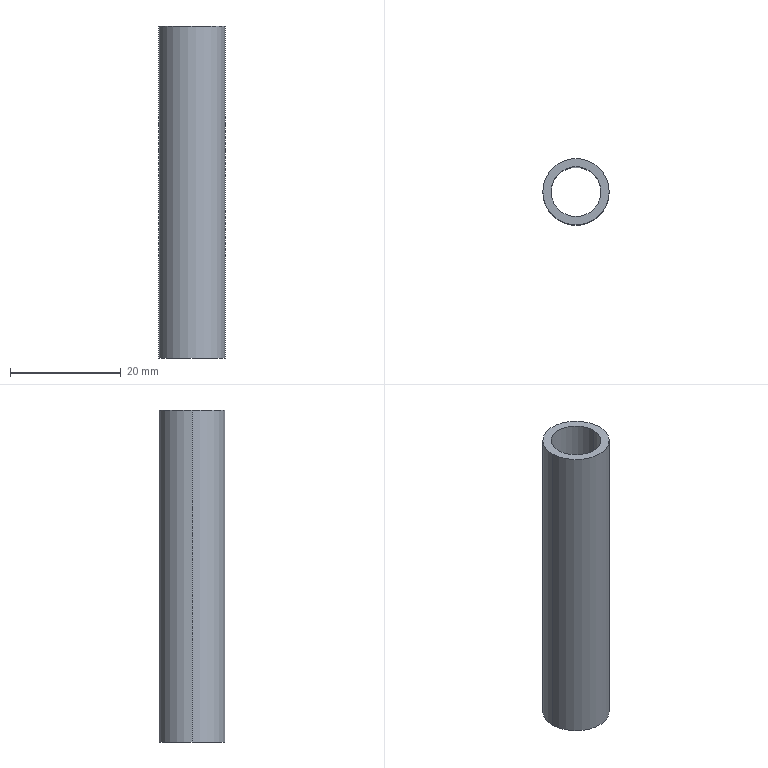Part | STEP file | 750038133 | 1 solid | 6 faces | box 12 x 12 x 60 mm | volume 2969 mm3 | cylinder 4 | plane 2 | commonest cylinder face diameters 9 x2 12 x2
STEP:
#1=CARTESIAN_POINT('',(-6.,0.,60.));
#2=VERTEX_POINT('',#1);
#3=CARTESIAN_POINT('',(6.,0.,60.));
#4=VERTEX_POINT('',#3);
#5=CARTESIAN_POINT('',(0.,0.,60.));
#6=DIRECTION('',(0.,0.,-1.));
#7=DIRECTION('',(-1.,0.,0.));
#8=AXIS2_PLACEMENT_3D('',#5,#6,#7);
#9=CIRCLE('',#8,6.);
#10=EDGE_CURVE('',#2,#4,#9,.T.);
#11=ORIENTED_EDGE('',*,*,#10,.T.);
#12=CARTESIAN_POINT('',(6.,0.,0.));
#13=VERTEX_POINT('',#12);
#14=CARTESIAN_POINT('',(6.,0.,60.));
#15=DIRECTION('',(0.,0.,-1.));
#16=VECTOR('',#15,1000.);
#17=LINE('',#14,#16);
#18=EDGE_CURVE('',#4,#13,#17,.T.);
#19=ORIENTED_EDGE('',*,*,#18,.T.);
#20=CARTESIAN_POINT('',(-6.,0.,0.));
#21=VERTEX_POINT('',#20);
#22=CARTESIAN_POINT('',(0.,0.,0.));
#23=DIRECTION('',(0.,0.,1.));
#24=DIRECTION('',(-1.,0.,0.));
#25=AXIS2_PLACEMENT_3D('',#22,#23,#24);
#26=CIRCLE('',#25,6.);
#27=EDGE_CURVE('',#13,#21,#26,.T.);
#28=ORIENTED_EDGE('',*,*,#27,.T.);
#29=CARTESIAN_POINT('',(-6.,0.,60.));
#30=DIRECTION('',(0.,0.,-1.));
#31=VECTOR('',#30,1000.);
#32=LINE('',#29,#31);
#33=EDGE_CURVE('',#2,#21,#32,.T.);
#34=ORIENTED_EDGE('',*,*,#33,.F.);
#35=EDGE_LOOP('',(#11,#19,#28,#34));
#36=FACE_OUTER_BOUND('',#35,.T.);
#37=CARTESIAN_POINT('',(0.,0.,60.));
#38=DIRECTION('',(0.,0.,-1.));
#39=DIRECTION('',(-1.,0.,0.));
#40=AXIS2_PLACEMENT_3D('',#37,#38,#39);
#41=CYLINDRICAL_SURFACE('',#40,6.);
#42=ADVANCED_FACE('',(#36),#41,.T.);
#43=CARTESIAN_POINT('',(4.5,0.,60.));
#44=VERTEX_POINT('',#43);
#45=CARTESIAN_POINT('',(-4.5,0.,60.));
#46=VERTEX_POINT('',#45);
#47=CARTESIAN_POINT('',(0.,0.,60.));
#48=DIRECTION('',(0.,0.,-1.));
#49=DIRECTION('',(-1.,0.,0.));
#50=AXIS2_PLACEMENT_3D('',#47,#48,#49);
#51=CIRCLE('',#50,4.5);
#52=EDGE_CURVE('',#44,#46,#51,.T.);
#53=ORIENTED_EDGE('',*,*,#52,.F.);
#54=CARTESIAN_POINT('',(4.5,0.,0.));
#55=VERTEX_POINT('',#54);
#56=CARTESIAN_POINT('',(4.5,0.,60.));
#57=DIRECTION('',(0.,0.,-1.));
#58=VECTOR('',#57,1000.);
#59=LINE('',#56,#58);
#60=EDGE_CURVE('',#44,#55,#59,.T.);
#61=ORIENTED_EDGE('',*,*,#60,.T.);
#62=CARTESIAN_POINT('',(-4.5,0.,0.));
#63=VERTEX_POINT('',#62);
#64=CARTESIAN_POINT('',(0.,0.,0.));
#65=DIRECTION('',(0.,0.,-1.));
#66=DIRECTION('',(-1.,0.,0.));
#67=AXIS2_PLACEMENT_3D('',#64,#65,#66);
#68=CIRCLE('',#67,4.5);
#69=EDGE_CURVE('',#55,#63,#68,.T.);
#70=ORIENTED_EDGE('',*,*,#69,.T.);
#71=CARTESIAN_POINT('',(-4.5,0.,60.));
#72=DIRECTION('',(0.,0.,-1.));
#73=VECTOR('',#72,1000.);
#74=LINE('',#71,#73);
#75=EDGE_CURVE('',#46,#63,#74,.T.);
#76=ORIENTED_EDGE('',*,*,#75,.F.);
#77=EDGE_LOOP('',(#53,#61,#70,#76));
#78=FACE_OUTER_BOUND('',#77,.T.);
#79=CARTESIAN_POINT('',(0.,0.,60.));
#80=DIRECTION('',(0.,0.,-1.));
#81=DIRECTION('',(-1.,0.,0.));
#82=AXIS2_PLACEMENT_3D('',#79,#80,#81);
#83=CYLINDRICAL_SURFACE('',#82,4.5);
#84=ADVANCED_FACE('',(#78),#83,.F.);
#85=ORIENTED_EDGE('',*,*,#18,.F.);
#86=CARTESIAN_POINT('',(0.,0.,60.));
#87=DIRECTION('',(0.,0.,-1.));
#88=DIRECTION('',(-1.,0.,0.));
#89=AXIS2_PLACEMENT_3D('',#86,#87,#88);
#90=CIRCLE('',#89,6.);
#91=EDGE_CURVE('',#4,#2,#90,.T.);
#92=ORIENTED_EDGE('',*,*,#91,.T.);
#93=ORIENTED_EDGE('',*,*,#33,.T.);
#94=CARTESIAN_POINT('',(0.,0.,0.));
#95=DIRECTION('',(0.,0.,1.));
#96=DIRECTION('',(-1.,0.,0.));
#97=AXIS2_PLACEMENT_3D('',#94,#95,#96);
#98=CIRCLE('',#97,6.);
#99=EDGE_CURVE('',#21,#13,#98,.T.);
#100=ORIENTED_EDGE('',*,*,#99,.T.);
#101=EDGE_LOOP('',(#85,#92,#93,#100));
#102=FACE_OUTER_BOUND('',#101,.T.);
#103=CARTESIAN_POINT('',(0.,0.,60.));
#104=DIRECTION('',(0.,0.,-1.));
#105=DIRECTION('',(-1.,0.,0.));
#106=AXIS2_PLACEMENT_3D('',#103,#104,#105);
#107=CYLINDRICAL_SURFACE('',#106,6.);
#108=ADVANCED_FACE('',(#102),#107,.T.);
#109=CARTESIAN_POINT('',(0.,0.,0.));
#110=DIRECTION('',(0.,0.,-1.));
#111=DIRECTION('',(-1.,0.,0.));
#112=AXIS2_PLACEMENT_3D('',#109,#110,#111);
#113=CIRCLE('',#112,4.5);
#114=EDGE_CURVE('',#63,#55,#113,.T.);
#115=ORIENTED_EDGE('',*,*,#114,.F.);
#116=ORIENTED_EDGE('',*,*,#69,.F.);
#117=EDGE_LOOP('',(#115,#116));
#118=FACE_BOUND('',#117,.T.);
#119=ORIENTED_EDGE('',*,*,#99,.F.);
#120=ORIENTED_EDGE('',*,*,#27,.F.);
#121=EDGE_LOOP('',(#119,#120));
#122=FACE_OUTER_BOUND('',#121,.T.);
#123=CARTESIAN_POINT('',(0.,0.,0.));
#124=DIRECTION('',(0.,0.,1.));
#125=DIRECTION('',(1.,0.,0.));
#126=AXIS2_PLACEMENT_3D('',#123,#124,#125);
#127=PLANE('',#126);
#128=ADVANCED_FACE('',(#118,#122),#127,.F.);
#129=CARTESIAN_POINT('',(0.,0.,60.));
#130=DIRECTION('',(0.,0.,-1.));
#131=DIRECTION('',(-1.,0.,0.));
#132=AXIS2_PLACEMENT_3D('',#129,#130,#131);
#133=CIRCLE('',#132,4.5);
#134=EDGE_CURVE('',#46,#44,#133,.T.);
#135=ORIENTED_EDGE('',*,*,#134,.T.);
#136=ORIENTED_EDGE('',*,*,#52,.T.);
#137=EDGE_LOOP('',(#135,#136));
#138=FACE_BOUND('',#137,.T.);
#139=ORIENTED_EDGE('',*,*,#10,.F.);
#140=ORIENTED_EDGE('',*,*,#91,.F.);
#141=EDGE_LOOP('',(#139,#140));
#142=FACE_OUTER_BOUND('',#141,.T.);
#143=CARTESIAN_POINT('',(0.,0.,60.));
#144=DIRECTION('',(0.,0.,1.));
#145=DIRECTION('',(1.,0.,0.));
#146=AXIS2_PLACEMENT_3D('',#143,#144,#145);
#147=PLANE('',#146);
#148=ADVANCED_FACE('',(#138,#142),#147,.T.);
#149=ORIENTED_EDGE('',*,*,#60,.F.);
#150=ORIENTED_EDGE('',*,*,#134,.F.);
#151=ORIENTED_EDGE('',*,*,#75,.T.);
#152=ORIENTED_EDGE('',*,*,#114,.T.);
#153=EDGE_LOOP('',(#149,#150,#151,#152));
#154=FACE_OUTER_BOUND('',#153,.T.);
#155=CARTESIAN_POINT('',(0.,0.,60.));
#156=DIRECTION('',(0.,0.,-1.));
#157=DIRECTION('',(-1.,0.,0.));
#158=AXIS2_PLACEMENT_3D('',#155,#156,#157);
#159=CYLINDRICAL_SURFACE('',#158,4.5);
#160=ADVANCED_FACE('',(#154),#159,.F.);
#161=CLOSED_SHELL('',(#42,#84,#108,#128,#148,#160));
#162=MANIFOLD_SOLID_BREP('',#161);
#163=CARTESIAN_POINT('',(0.,0.,0.));
#164=DIRECTION('',(0.,0.,1.));
#165=DIRECTION('',(1.,0.,0.));
#166=AXIS2_PLACEMENT_3D('',#163,#164,#165);
#167=(LENGTH_UNIT()NAMED_UNIT(*)SI_UNIT(.MILLI.,.METRE.));
#168=UNCERTAINTY_MEASURE_WITH_UNIT(LENGTH_MEASURE(0.00001),#167,'','');
#169=(NAMED_UNIT(*)PLANE_ANGLE_UNIT()SI_UNIT($,.RADIAN.));
#170=(NAMED_UNIT(*)SI_UNIT($,.STERADIAN.)SOLID_ANGLE_UNIT());
#171=(GEOMETRIC_REPRESENTATION_CONTEXT(3)GLOBAL_UNCERTAINTY_ASSIGNED_CONTEXT((#168))GLOBAL_UNIT_ASSIGNED_CONTEXT((#167,#169,#170))REPRESENTATION_CONTEXT('',''));
#172=ADVANCED_BREP_SHAPE_REPRESENTATION('',(#162,#166),#171);